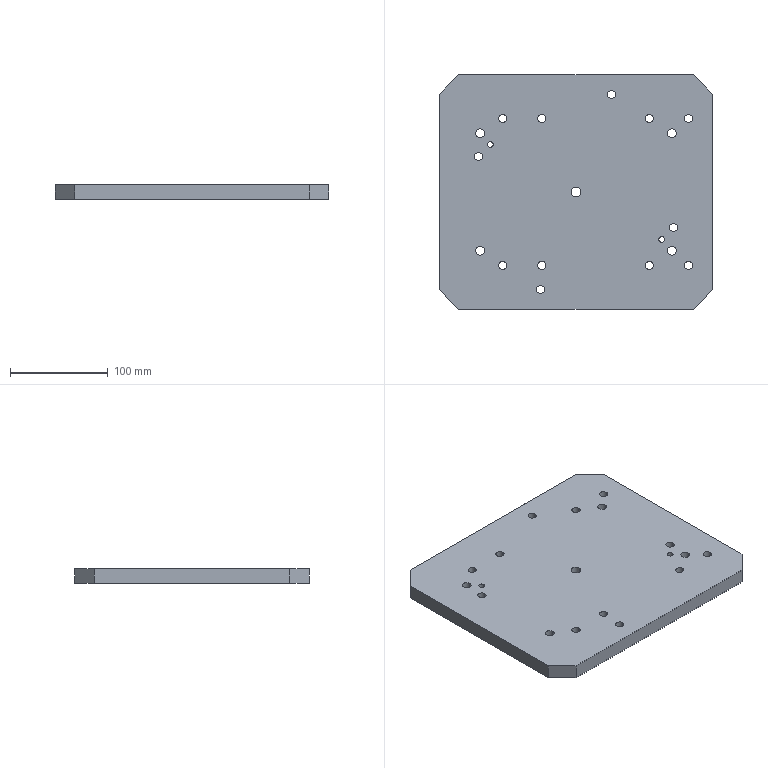Part | STEP file | ASND-0110-Body 1-1 | 1 solid | 60 faces | box 280 x 240 x 15 mm | volume 976987 mm3 | cylinder 46 | plane 14 | commonest cylinder face diameters 8.376 x24 9 x8 14 x8 6 x4 10 x2